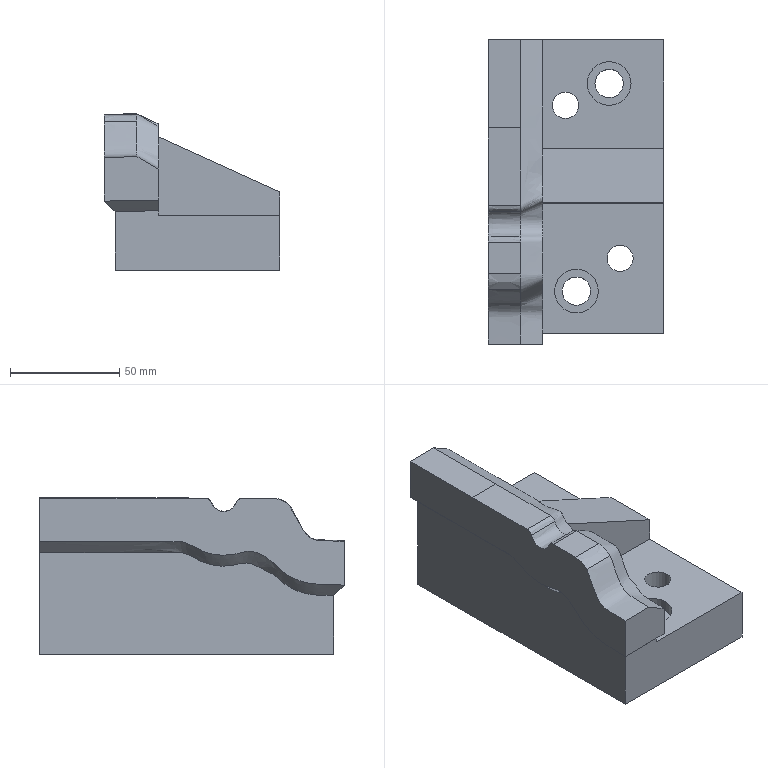Part | NX | features solid 2 | 1 solid | 32 faces | box 80.373 x 139.38 x 71.521 mm | volume 404054 mm3 | plane 13 | spline 13 | cylinder 6 | commonest cylinder face diameters 12 x2 13 x2 20 x2